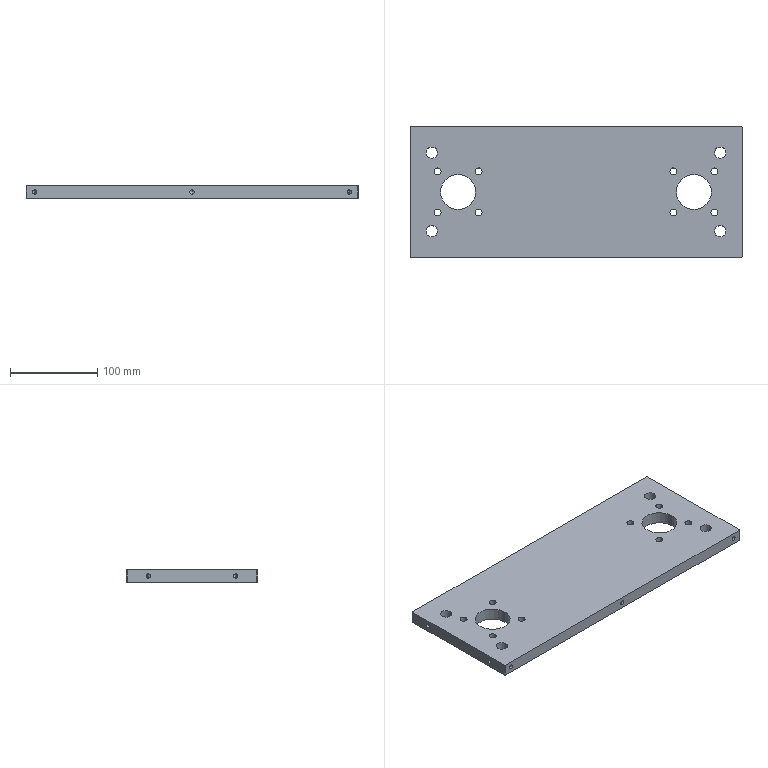Part | SolidWorks | features HoleWzd 6, 3DProfileFeature 2, Chamfer 1, Extrusion 1, ICE 1, LPattern 1 | 1 solid | 78 faces | box 380 x 150 x 14 mm | volume 746680 mm3 | cylinder 48 | cone 20 | plane 10 | commonest cylinder face diameters 5 x20 8 x16 13 x8 40 x4